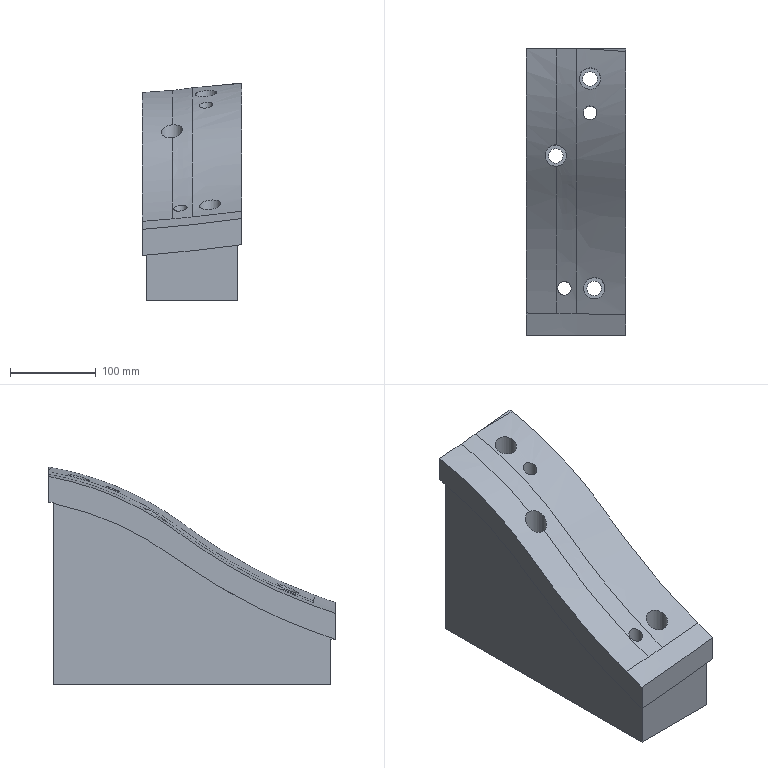Part | NX | features solid 2 | 1 solid | 37 faces | box 116.651 x 335.001 x 254.783 mm | volume 5770313 mm3 | plane 15 | spline 12 | cylinder 10 | commonest cylinder face diameters 25 x5 17 x3 16 x2